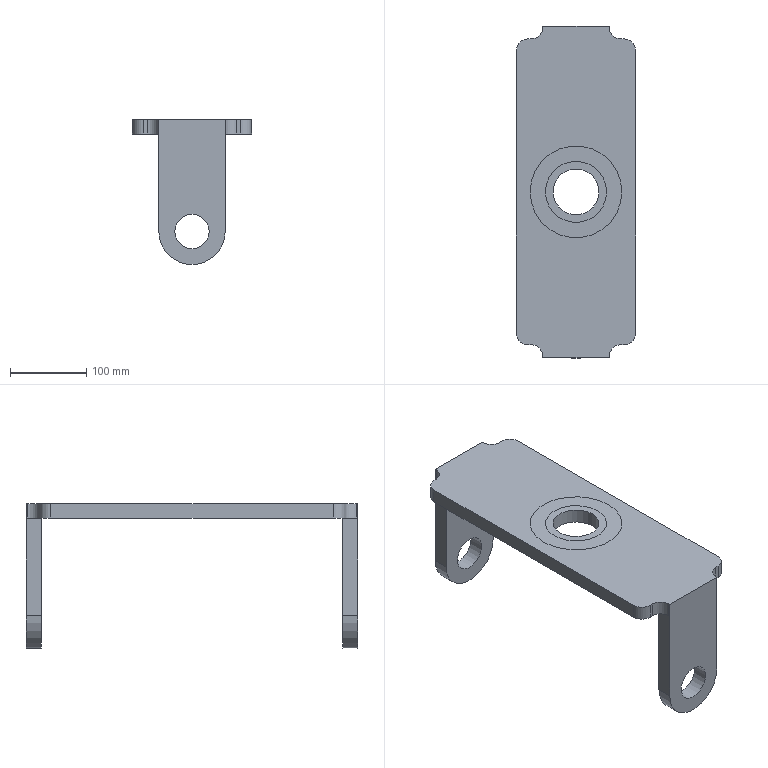Part | NX | features BREP 3 | 3 solids | 37 faces | box 156 x 434 x 190 mm | volume 1687057 mm3 | plane 20 | cylinder 17 | commonest cylinder face diameters 30 x8 45 x2 80 x2 87 x2 120 x2 60 x1
STEP:
#1=CARTESIAN_POINT('',(43.5,215.,19.));
#2=VERTEX_POINT('',#1);
#3=CARTESIAN_POINT('',(43.5,217.,19.));
#4=VERTEX_POINT('',#3);
#5=CARTESIAN_POINT('',(43.5,217.,19.));
#6=DIRECTION('',(0.,1.,0.));
#7=VECTOR('',#6,1000.);
#8=LINE('',#5,#7);
#9=EDGE_CURVE('',#2,#4,#8,.T.);
#10=ORIENTED_EDGE('',*,*,#9,.F.);
#11=CARTESIAN_POINT('',(43.5,215.,0.));
#12=VERTEX_POINT('',#11);
#13=CARTESIAN_POINT('',(43.5,215.,0.));
#14=DIRECTION('',(0.,0.,-1.));
#15=VECTOR('',#14,1000.);
#16=LINE('',#13,#15);
#17=EDGE_CURVE('',#2,#12,#16,.T.);
#18=ORIENTED_EDGE('',*,*,#17,.T.);
#19=CARTESIAN_POINT('',(43.5,197.,0.));
#20=VERTEX_POINT('',#19);
#21=CARTESIAN_POINT('',(43.5,217.,0.));
#22=DIRECTION('',(0.,-1.,0.));
#23=VECTOR('',#22,1000.);
#24=LINE('',#21,#23);
#25=EDGE_CURVE('',#12,#20,#24,.T.);
#26=ORIENTED_EDGE('',*,*,#25,.T.);
#27=CARTESIAN_POINT('',(43.5,197.,-127.5));
#28=VERTEX_POINT('',#27);
#29=CARTESIAN_POINT('',(43.5,197.,0.));
#30=DIRECTION('',(0.,0.,1.));
#31=VECTOR('',#30,1000.);
#32=LINE('',#29,#31);
#33=EDGE_CURVE('',#28,#20,#32,.T.);
#34=ORIENTED_EDGE('',*,*,#33,.F.);
#35=CARTESIAN_POINT('',(43.5,217.,-127.5));
#36=VERTEX_POINT('',#35);
#37=CARTESIAN_POINT('',(43.5,217.,-127.5));
#38=DIRECTION('',(0.,1.,0.));
#39=VECTOR('',#38,1000.);
#40=LINE('',#37,#39);
#41=EDGE_CURVE('',#28,#36,#40,.T.);
#42=ORIENTED_EDGE('',*,*,#41,.T.);
#43=CARTESIAN_POINT('',(43.5,217.,0.));
#44=DIRECTION('',(0.,0.,1.));
#45=VECTOR('',#44,1000.);
#46=LINE('',#43,#45);
#47=EDGE_CURVE('',#36,#4,#46,.T.);
#48=ORIENTED_EDGE('',*,*,#47,.T.);
#49=EDGE_LOOP('',(#10,#18,#26,#34,#42,#48));
#50=FACE_BOUND('',#49,.T.);
#51=CARTESIAN_POINT('',(43.5,217.,0.));
#52=DIRECTION('',(1.,0.,0.));
#53=DIRECTION('',(0.,0.,1.));
#54=AXIS2_PLACEMENT_3D('',#51,#52,#53);
#55=PLANE('',#54);
#56=ADVANCED_FACE('',(#50),#55,.T.);
#57=CARTESIAN_POINT('',(-43.5,197.,0.));
#58=VERTEX_POINT('',#57);
#59=CARTESIAN_POINT('',(-43.5,215.,0.));
#60=VERTEX_POINT('',#59);
#61=CARTESIAN_POINT('',(-43.5,217.,0.));
#62=DIRECTION('',(0.,1.,0.));
#63=VECTOR('',#62,1000.);
#64=LINE('',#61,#63);
#65=EDGE_CURVE('',#58,#60,#64,.T.);
#66=ORIENTED_EDGE('',*,*,#65,.T.);
#67=CARTESIAN_POINT('',(-43.5,215.,19.));
#68=VERTEX_POINT('',#67);
#69=CARTESIAN_POINT('',(-43.5,215.,-127.5));
#70=DIRECTION('',(0.,0.,1.));
#71=VECTOR('',#70,1000.);
#72=LINE('',#69,#71);
#73=EDGE_CURVE('',#60,#68,#72,.T.);
#74=ORIENTED_EDGE('',*,*,#73,.T.);
#75=CARTESIAN_POINT('',(-43.5,217.,19.));
#76=VERTEX_POINT('',#75);
#77=CARTESIAN_POINT('',(-43.5,217.,19.));
#78=DIRECTION('',(0.,1.,0.));
#79=VECTOR('',#78,1000.);
#80=LINE('',#77,#79);
#81=EDGE_CURVE('',#68,#76,#80,.T.);
#82=ORIENTED_EDGE('',*,*,#81,.T.);
#83=CARTESIAN_POINT('',(-43.5,217.,-127.5));
#84=VERTEX_POINT('',#83);
#85=CARTESIAN_POINT('',(-43.5,217.,-127.5));
#86=DIRECTION('',(0.,0.,-1.));
#87=VECTOR('',#86,1000.);
#88=LINE('',#85,#87);
#89=EDGE_CURVE('',#76,#84,#88,.T.);
#90=ORIENTED_EDGE('',*,*,#89,.T.);
#91=CARTESIAN_POINT('',(-43.5,197.,-127.5));
#92=VERTEX_POINT('',#91);
#93=CARTESIAN_POINT('',(-43.5,217.,-127.5));
#94=DIRECTION('',(0.,1.,0.));
#95=VECTOR('',#94,1000.);
#96=LINE('',#93,#95);
#97=EDGE_CURVE('',#92,#84,#96,.T.);
#98=ORIENTED_EDGE('',*,*,#97,.F.);
#99=CARTESIAN_POINT('',(-43.5,197.,-127.5));
#100=DIRECTION('',(0.,0.,-1.));
#101=VECTOR('',#100,1000.);
#102=LINE('',#99,#101);
#103=EDGE_CURVE('',#58,#92,#102,.T.);
#104=ORIENTED_EDGE('',*,*,#103,.F.);
#105=EDGE_LOOP('',(#66,#74,#82,#90,#98,#104));
#106=FACE_BOUND('',#105,.T.);
#107=CARTESIAN_POINT('',(-43.5,217.,-127.5));
#108=DIRECTION('',(-1.,0.,0.));
#109=DIRECTION('',(0.,0.,-1.));
#110=AXIS2_PLACEMENT_3D('',#107,#108,#109);
#111=PLANE('',#110);
#112=ADVANCED_FACE('',(#106),#111,.T.);
#113=CARTESIAN_POINT('',(22.5,197.,-127.5));
#114=VERTEX_POINT('',#113);
#115=CARTESIAN_POINT('',(0.,197.,-127.5));
#116=DIRECTION('',(0.,-1.,0.));
#117=DIRECTION('',(1.,0.,0.));
#118=AXIS2_PLACEMENT_3D('',#115,#116,#117);
#119=CIRCLE('',#118,22.5);
#120=EDGE_CURVE('',#114,#114,#119,.T.);
#121=ORIENTED_EDGE('',*,*,#120,.F.);
#122=EDGE_LOOP('',(#121));
#123=FACE_BOUND('',#122,.T.);
#124=ORIENTED_EDGE('',*,*,#33,.T.);
#125=CARTESIAN_POINT('',(0.,197.,0.));
#126=DIRECTION('',(-1.,0.,0.));
#127=VECTOR('',#126,1000.);
#128=LINE('',#125,#127);
#129=EDGE_CURVE('',#20,#58,#128,.T.);
#130=ORIENTED_EDGE('',*,*,#129,.T.);
#131=ORIENTED_EDGE('',*,*,#103,.T.);
#132=CARTESIAN_POINT('',(0.,197.,-127.5));
#133=DIRECTION('',(0.,-1.,0.));
#134=DIRECTION('',(1.,0.,0.));
#135=AXIS2_PLACEMENT_3D('',#132,#133,#134);
#136=CIRCLE('',#135,43.5);
#137=EDGE_CURVE('',#92,#28,#136,.T.);
#138=ORIENTED_EDGE('',*,*,#137,.T.);
#139=EDGE_LOOP('',(#124,#130,#131,#138));
#140=FACE_BOUND('',#139,.T.);
#141=CARTESIAN_POINT('',(0.,197.,-127.5));
#142=DIRECTION('',(0.,-1.,0.));
#143=DIRECTION('',(0.,0.,-1.));
#144=AXIS2_PLACEMENT_3D('',#141,#142,#143);
#145=PLANE('',#144);
#146=ADVANCED_FACE('',(#123,#140),#145,.T.);
#147=ORIENTED_EDGE('',*,*,#137,.F.);
#148=ORIENTED_EDGE('',*,*,#97,.T.);
#149=CARTESIAN_POINT('',(0.,217.,-127.5));
#150=DIRECTION('',(0.,-1.,0.));
#151=DIRECTION('',(1.,0.,0.));
#152=AXIS2_PLACEMENT_3D('',#149,#150,#151);
#153=CIRCLE('',#152,43.5);
#154=EDGE_CURVE('',#84,#36,#153,.T.);
#155=ORIENTED_EDGE('',*,*,#154,.T.);
#156=ORIENTED_EDGE('',*,*,#41,.F.);
#157=EDGE_LOOP('',(#147,#148,#155,#156));
#158=FACE_BOUND('',#157,.T.);
#159=CARTESIAN_POINT('',(0.,217.,-127.5));
#160=DIRECTION('',(0.,-1.,0.));
#161=DIRECTION('',(0.,0.,-1.));
#162=AXIS2_PLACEMENT_3D('',#159,#160,#161);
#163=CYLINDRICAL_SURFACE('',#162,43.5);
#164=ADVANCED_FACE('',(#158),#163,.T.);
#165=CARTESIAN_POINT('',(60.,0.,19.));
#166=VERTEX_POINT('',#165);
#167=CARTESIAN_POINT('',(0.,0.,19.));
#168=DIRECTION('',(0.,0.,1.));
#169=DIRECTION('',(1.,0.,0.));
#170=AXIS2_PLACEMENT_3D('',#167,#168,#169);
#171=CIRCLE('',#170,60.);
#172=EDGE_CURVE('',#166,#166,#171,.T.);
#173=ORIENTED_EDGE('',*,*,#172,.F.);
#174=EDGE_LOOP('',(#173));
#175=FACE_BOUND('',#174,.T.);
#176=CARTESIAN_POINT('',(-78.,185.,19.));
#177=VERTEX_POINT('',#176);
#178=CARTESIAN_POINT('',(-78.,-185.,19.));
#179=VERTEX_POINT('',#178);
#180=CARTESIAN_POINT('',(-78.,175.,19.));
#181=DIRECTION('',(0.,-1.,0.));
#182=VECTOR('',#181,1000.);
#183=LINE('',#180,#182);
#184=EDGE_CURVE('',#177,#179,#183,.T.);
#185=ORIENTED_EDGE('',*,*,#184,.T.);
#186=CARTESIAN_POINT('',(-63.,-200.,19.));
#187=VERTEX_POINT('',#186);
#188=CARTESIAN_POINT('',(-63.,-185.,19.));
#189=DIRECTION('',(0.,0.,1.));
#190=DIRECTION('',(1.,0.,0.));
#191=AXIS2_PLACEMENT_3D('',#188,#189,#190);
#192=CIRCLE('',#191,15.);
#193=EDGE_CURVE('',#179,#187,#192,.T.);
#194=ORIENTED_EDGE('',*,*,#193,.T.);
#195=CARTESIAN_POINT('',(-58.5,-200.,19.));
#196=VERTEX_POINT('',#195);
#197=CARTESIAN_POINT('',(-48.,-200.,19.));
#198=DIRECTION('',(1.,0.,0.));
#199=VECTOR('',#198,1000.);
#200=LINE('',#197,#199);
#201=EDGE_CURVE('',#187,#196,#200,.T.);
#202=ORIENTED_EDGE('',*,*,#201,.T.);
#203=CARTESIAN_POINT('',(-43.5,-215.,19.));
#204=VERTEX_POINT('',#203);
#205=CARTESIAN_POINT('',(-58.5,-215.,19.));
#206=DIRECTION('',(0.,0.,-1.));
#207=DIRECTION('',(1.,0.,0.));
#208=AXIS2_PLACEMENT_3D('',#205,#206,#207);
#209=CIRCLE('',#208,15.);
#210=EDGE_CURVE('',#196,#204,#209,.T.);
#211=ORIENTED_EDGE('',*,*,#210,.T.);
#212=CARTESIAN_POINT('',(-43.5,-217.,19.));
#213=VERTEX_POINT('',#212);
#214=CARTESIAN_POINT('',(-43.5,-217.,19.));
#215=DIRECTION('',(0.,1.,0.));
#216=VECTOR('',#215,1000.);
#217=LINE('',#214,#216);
#218=EDGE_CURVE('',#213,#204,#217,.T.);
#219=ORIENTED_EDGE('',*,*,#218,.F.);
#220=CARTESIAN_POINT('',(43.5,-217.,19.));
#221=VERTEX_POINT('',#220);
#222=CARTESIAN_POINT('',(0.,-217.,19.));
#223=DIRECTION('',(1.,0.,0.));
#224=VECTOR('',#223,1000.);
#225=LINE('',#222,#224);
#226=EDGE_CURVE('',#213,#221,#225,.T.);
#227=ORIENTED_EDGE('',*,*,#226,.T.);
#228=CARTESIAN_POINT('',(43.5,-215.,19.));
#229=VERTEX_POINT('',#228);
#230=CARTESIAN_POINT('',(43.5,-217.,19.));
#231=DIRECTION('',(0.,1.,0.));
#232=VECTOR('',#231,1000.);
#233=LINE('',#230,#232);
#234=EDGE_CURVE('',#221,#229,#233,.T.);
#235=ORIENTED_EDGE('',*,*,#234,.T.);
#236=CARTESIAN_POINT('',(58.5,-200.,19.));
#237=VERTEX_POINT('',#236);
#238=CARTESIAN_POINT('',(58.5,-215.,19.));
#239=DIRECTION('',(0.,0.,-1.));
#240=DIRECTION('',(1.,0.,0.));
#241=AXIS2_PLACEMENT_3D('',#238,#239,#240);
#242=CIRCLE('',#241,15.);
#243=EDGE_CURVE('',#229,#237,#242,.T.);
#244=ORIENTED_EDGE('',*,*,#243,.T.);
#245=CARTESIAN_POINT('',(63.,-200.,19.));
#246=VERTEX_POINT('',#245);
#247=CARTESIAN_POINT('',(-48.,-200.,19.));
#248=DIRECTION('',(1.,0.,0.));
#249=VECTOR('',#248,1000.);
#250=LINE('',#247,#249);
#251=EDGE_CURVE('',#237,#246,#250,.T.);
#252=ORIENTED_EDGE('',*,*,#251,.T.);
#253=CARTESIAN_POINT('',(78.,-185.,19.));
#254=VERTEX_POINT('',#253);
#255=CARTESIAN_POINT('',(63.,-185.,19.));
#256=DIRECTION('',(0.,0.,1.));
#257=DIRECTION('',(1.,0.,0.));
#258=AXIS2_PLACEMENT_3D('',#255,#256,#257);
#259=CIRCLE('',#258,15.);
#260=EDGE_CURVE('',#246,#254,#259,.T.);
#261=ORIENTED_EDGE('',*,*,#260,.T.);
#262=CARTESIAN_POINT('',(78.,185.,19.));
#263=VERTEX_POINT('',#262);
#264=CARTESIAN_POINT('',(78.,-175.,19.));
#265=DIRECTION('',(0.,1.,0.));
#266=VECTOR('',#265,1000.);
#267=LINE('',#264,#266);
#268=EDGE_CURVE('',#254,#263,#267,.T.);
#269=ORIENTED_EDGE('',*,*,#268,.T.);
#270=CARTESIAN_POINT('',(63.,200.,19.));
#271=VERTEX_POINT('',#270);
#272=CARTESIAN_POINT('',(63.,185.,19.));
#273=DIRECTION('',(0.,0.,1.));
#274=DIRECTION('',(1.,0.,0.));
#275=AXIS2_PLACEMENT_3D('',#272,#273,#274);
#276=CIRCLE('',#275,15.);
#277=EDGE_CURVE('',#263,#271,#276,.T.);
#278=ORIENTED_EDGE('',*,*,#277,.T.);
#279=CARTESIAN_POINT('',(58.5,200.,19.));
#280=VERTEX_POINT('',#279);
#281=CARTESIAN_POINT('',(-48.,200.,19.));
#282=DIRECTION('',(-1.,0.,0.));
#283=VECTOR('',#282,1000.);
#284=LINE('',#281,#283);
#285=EDGE_CURVE('',#271,#280,#284,.T.);
#286=ORIENTED_EDGE('',*,*,#285,.T.);
#287=CARTESIAN_POINT('',(58.5,215.,19.));
#288=DIRECTION('',(0.,0.,-1.));
#289=DIRECTION('',(1.,0.,0.));
#290=AXIS2_PLACEMENT_3D('',#287,#288,#289);
#291=CIRCLE('',#290,15.);
#292=EDGE_CURVE('',#280,#2,#291,.T.);
#293=ORIENTED_EDGE('',*,*,#292,.T.);
#294=ORIENTED_EDGE('',*,*,#9,.T.);
#295=CARTESIAN_POINT('',(0.,217.,19.));
#296=DIRECTION('',(-1.,0.,0.));
#297=VECTOR('',#296,1000.);
#298=LINE('',#295,#297);
#299=EDGE_CURVE('',#4,#76,#298,.T.);
#300=ORIENTED_EDGE('',*,*,#299,.T.);
#301=ORIENTED_EDGE('',*,*,#81,.F.);
#302=CARTESIAN_POINT('',(-58.5,200.,19.));
#303=VERTEX_POINT('',#302);
#304=CARTESIAN_POINT('',(-58.5,215.,19.));
#305=DIRECTION('',(0.,0.,-1.));
#306=DIRECTION('',(1.,0.,0.));
#307=AXIS2_PLACEMENT_3D('',#304,#305,#306);
#308=CIRCLE('',#307,15.);
#309=EDGE_CURVE('',#68,#303,#308,.T.);
#310=ORIENTED_EDGE('',*,*,#309,.T.);
#311=CARTESIAN_POINT('',(-63.,200.,19.));
#312=VERTEX_POINT('',#311);
#313=CARTESIAN_POINT('',(-48.,200.,19.));
#314=DIRECTION('',(-1.,0.,0.));
#315=VECTOR('',#314,1000.);
#316=LINE('',#313,#315);
#317=EDGE_CURVE('',#303,#312,#316,.T.);
#318=ORIENTED_EDGE('',*,*,#317,.T.);
#319=CARTESIAN_POINT('',(-63.,185.,19.));
#320=DIRECTION('',(0.,0.,1.));
#321=DIRECTION('',(1.,0.,0.));
#322=AXIS2_PLACEMENT_3D('',#319,#320,#321);
#323=CIRCLE('',#322,15.);
#324=EDGE_CURVE('',#312,#177,#323,.T.);
#325=ORIENTED_EDGE('',*,*,#324,.T.);
#326=EDGE_LOOP('',(#185,#194,#202,#211,#219,#227,#235,#244,#252,#261,#269,#278,#286,#293,#294,#300,#301,#310,#318,#325));
#327=FACE_BOUND('',#326,.T.);
#328=CARTESIAN_POINT('',(-43.5,217.,19.));
#329=DIRECTION('',(0.,0.,1.));
#330=DIRECTION('',(-1.,0.,0.));
#331=AXIS2_PLACEMENT_3D('',#328,#329,#330);
#332=PLANE('',#331);
#333=ADVANCED_FACE('',(#175,#327),#332,.T.);
#334=CARTESIAN_POINT('',(22.5,217.,-127.5));
#335=VERTEX_POINT('',#334);
#336=CARTESIAN_POINT('',(0.,217.,-127.5));
#337=DIRECTION('',(0.,-1.,0.));
#338=DIRECTION('',(1.,0.,0.));
#339=AXIS2_PLACEMENT_3D('',#336,#337,#338);
#340=CIRCLE('',#339,22.5);
#341=EDGE_CURVE('',#335,#335,#340,.T.);
#342=ORIENTED_EDGE('',*,*,#341,.F.);
#343=EDGE_LOOP('',(#342));
#344=FACE_BOUND('',#343,.T.);
#345=ORIENTED_EDGE('',*,*,#120,.T.);
#346=EDGE_LOOP('',(#345));
#347=FACE_BOUND('',#346,.T.);
#348=CARTESIAN_POINT('',(0.,217.,-127.5));
#349=DIRECTION('',(0.,-1.,0.));
#350=DIRECTION('',(0.,0.,-1.));
#351=AXIS2_PLACEMENT_3D('',#348,#349,#350);
#352=CYLINDRICAL_SURFACE('',#351,22.5);
#353=ADVANCED_FACE('',(#344,#347),#352,.F.);
#354=ORIENTED_EDGE('',*,*,#47,.F.);
#355=ORIENTED_EDGE('',*,*,#154,.F.);
#356=ORIENTED_EDGE('',*,*,#89,.F.);
#357=ORIENTED_EDGE('',*,*,#299,.F.);
#358=EDGE_LOOP('',(#354,#355,#356,#357));
#359=FACE_BOUND('',#358,.T.);
#360=ORIENTED_EDGE('',*,*,#341,.T.);
#361=EDGE_LOOP('',(#360));
#362=FACE_BOUND('',#361,.T.);
#363=CARTESIAN_POINT('',(0.,217.,-127.5));
#364=DIRECTION('',(0.,-1.,0.));
#365=DIRECTION('',(0.,0.,-1.));
#366=AXIS2_PLACEMENT_3D('',#363,#364,#365);
#367=PLANE('',#366);
#368=ADVANCED_FACE('',(#359,#362),#367,.F.);
#369=ORIENTED_EDGE('',*,*,#285,.F.);
#370=CARTESIAN_POINT('',(63.,200.,0.));
#371=VERTEX_POINT('',#370);
#372=CARTESIAN_POINT('',(63.,200.,19.));
#373=DIRECTION('',(0.,0.,-1.));
#374=VECTOR('',#373,1000.);
#375=LINE('',#372,#374);
#376=EDGE_CURVE('',#271,#371,#375,.T.);
#377=ORIENTED_EDGE('',*,*,#376,.T.);
#378=CARTESIAN_POINT('',(58.5,200.,0.));
#379=VERTEX_POINT('',#378);
#380=CARTESIAN_POINT('',(-48.,200.,0.));
#381=DIRECTION('',(-1.,0.,0.));
#382=VECTOR('',#381,1000.);
#383=LINE('',#380,#382);
#384=EDGE_CURVE('',#371,#379,#383,.T.);
#385=ORIENTED_EDGE('',*,*,#384,.T.);
#386=CARTESIAN_POINT('',(58.5,200.,19.));
#387=DIRECTION('',(0.,0.,1.));
#388=VECTOR('',#387,1000.);
#389=LINE('',#386,#388);
#390=EDGE_CURVE('',#379,#280,#389,.T.);
#391=ORIENTED_EDGE('',*,*,#390,.T.);
#392=EDGE_LOOP('',(#369,#377,#385,#391));
#393=FACE_BOUND('',#392,.T.);
#394=CARTESIAN_POINT('',(-48.,200.,19.));
#395=DIRECTION('',(0.,-1.,0.));
#396=DIRECTION('',(-1.,0.,0.));
#397=AXIS2_PLACEMENT_3D('',#394,#395,#396);
#398=PLANE('',#397);
#399=ADVANCED_FACE('',(#393),#398,.F.);
#400=CARTESIAN_POINT('',(58.5,-200.,0.));
#401=VERTEX_POINT('',#400);
#402=CARTESIAN_POINT('',(63.,-200.,0.));
#403=VERTEX_POINT('',#402);
#404=CARTESIAN_POINT('',(-48.,-200.,0.));
#405=DIRECTION('',(1.,0.,0.));
#406=VECTOR('',#405,1000.);
#407=LINE('',#404,#406);
#408=EDGE_CURVE('',#401,#403,#407,.T.);
#409=ORIENTED_EDGE('',*,*,#408,.T.);
#410=CARTESIAN_POINT('',(63.,-200.,19.));
#411=DIRECTION('',(0.,0.,1.));
#412=VECTOR('',#411,1000.);
#413=LINE('',#410,#412);
#414=EDGE_CURVE('',#403,#246,#413,.T.);
#415=ORIENTED_EDGE('',*,*,#414,.T.);
#416=ORIENTED_EDGE('',*,*,#251,.F.);
#417=CARTESIAN_POINT('',(58.5,-200.,19.));
#418=DIRECTION('',(0.,0.,-1.));
#419=VECTOR('',#418,1000.);
#420=LINE('',#417,#419);
#421=EDGE_CURVE('',#237,#401,#420,.T.);
#422=ORIENTED_EDGE('',*,*,#421,.T.);
#423=EDGE_LOOP('',(#409,#415,#416,#422));
#424=FACE_BOUND('',#423,.T.);
#425=CARTESIAN_POINT('',(-48.,-200.,19.));
#426=DIRECTION('',(0.,1.,0.));
#427=DIRECTION('',(0.,0.,-1.));
#428=AXIS2_PLACEMENT_3D('',#425,#426,#427);
#429=PLANE('',#428);
#430=ADVANCED_FACE('',(#424),#429,.F.);
#431=ORIENTED_EDGE('',*,*,#268,.F.);
#432=CARTESIAN_POINT('',(78.,-185.,0.));
#433=VERTEX_POINT('',#432);
#434=CARTESIAN_POINT('',(78.,-185.,19.));
#435=DIRECTION('',(0.,0.,-1.));
#436=VECTOR('',#435,1000.);
#437=LINE('',#434,#436);
#438=EDGE_CURVE('',#254,#433,#437,.T.);
#439=ORIENTED_EDGE('',*,*,#438,.T.);
#440=CARTESIAN_POINT('',(78.,185.,0.));
#441=VERTEX_POINT('',#440);
#442=CARTESIAN_POINT('',(78.,-175.,0.));
#443=DIRECTION('',(0.,1.,0.));
#444=VECTOR('',#443,1000.);
#445=LINE('',#442,#444);
#446=EDGE_CURVE('',#433,#441,#445,.T.);
#447=ORIENTED_EDGE('',*,*,#446,.T.);
#448=CARTESIAN_POINT('',(78.,185.,19.));
#449=DIRECTION('',(0.,0.,1.));
#450=VECTOR('',#449,1000.);
#451=LINE('',#448,#450);
#452=EDGE_CURVE('',#441,#263,#451,.T.);
#453=ORIENTED_EDGE('',*,*,#452,.T.);
#454=EDGE_LOOP('',(#431,#439,#447,#453));
#455=FACE_BOUND('',#454,.T.);
#456=CARTESIAN_POINT('',(78.,-175.,19.));
#457=DIRECTION('',(-1.,0.,0.));
#458=DIRECTION('',(0.,1.,0.));
#459=AXIS2_PLACEMENT_3D('',#456,#457,#458);
#460=PLANE('',#459);
#461=ADVANCED_FACE('',(#455),#460,.F.);
#462=CARTESIAN_POINT('',(-58.5,200.,0.));
#463=VERTEX_POINT('',#462);
#464=CARTESIAN_POINT('',(-63.,200.,0.));
#465=VERTEX_POINT('',#464);
#466=CARTESIAN_POINT('',(-48.,200.,0.));
#467=DIRECTION('',(-1.,0.,0.));
#468=VECTOR('',#467,1000.);
#469=LINE('',#466,#468);
#470=EDGE_CURVE('',#463,#465,#469,.T.);
#471=ORIENTED_EDGE('',*,*,#470,.T.);
#472=CARTESIAN_POINT('',(-63.,200.,19.));
#473=DIRECTION('',(0.,0.,1.));
#474=VECTOR('',#473,1000.);
#475=LINE('',#472,#474);
#476=EDGE_CURVE('',#465,#312,#475,.T.);
#477=ORIENTED_EDGE('',*,*,#476,.T.);
#478=ORIENTED_EDGE('',*,*,#317,.F.);
#479=CARTESIAN_POINT('',(-58.5,200.,19.));
#480=DIRECTION('',(0.,0.,-1.));
#481=VECTOR('',#480,1000.);
#482=LINE('',#479,#481);
#483=EDGE_CURVE('',#303,#463,#482,.T.);
#484=ORIENTED_EDGE('',*,*,#483,.T.);
#485=EDGE_LOOP('',(#471,#477,#478,#484));
#486=FACE_BOUND('',#485,.T.);
#487=CARTESIAN_POINT('',(-48.,200.,19.));
#488=DIRECTION('',(0.,-1.,0.));
#489=DIRECTION('',(-1.,0.,0.));
#490=AXIS2_PLACEMENT_3D('',#487,#488,#489);
#491=PLANE('',#490);
#492=ADVANCED_FACE('',(#486),#491,.F.);
#493=CARTESIAN_POINT('',(-78.,185.,0.));
#494=VERTEX_POINT('',#493);
#495=CARTESIAN_POINT('',(-78.,-185.,0.));
#496=VERTEX_POINT('',#495);
#497=CARTESIAN_POINT('',(-78.,175.,0.));
#498=DIRECTION('',(0.,-1.,0.));
#499=VECTOR('',#498,1000.);
#500=LINE('',#497,#499);
#501=EDGE_CURVE('',#494,#496,#500,.T.);
#502=ORIENTED_EDGE('',*,*,#501,.T.);
#503=CARTESIAN_POINT('',(-78.,-185.,19.));
#504=DIRECTION('',(0.,0.,1.));
#505=VECTOR('',#504,1000.);
#506=LINE('',#503,#505);
#507=EDGE_CURVE('',#496,#179,#506,.T.);
#508=ORIENTED_EDGE('',*,*,#507,.T.);
#509=ORIENTED_EDGE('',*,*,#184,.F.);
#510=CARTESIAN_POINT('',(-78.,185.,19.));
#511=DIRECTION('',(0.,0.,-1.));
#512=VECTOR('',#511,1000.);
#513=LINE('',#510,#512);
#514=EDGE_CURVE('',#177,#494,#513,.T.);
#515=ORIENTED_EDGE('',*,*,#514,.T.);
#516=EDGE_LOOP('',(#502,#508,#509,#515));
#517=FACE_BOUND('',#516,.T.);
#518=CARTESIAN_POINT('',(-78.,175.,19.));
#519=DIRECTION('',(1.,0.,0.));
#520=DIRECTION('',(0.,0.,1.));
#521=AXIS2_PLACEMENT_3D('',#518,#519,#520);
#522=PLANE('',#521);
#523=ADVANCED_FACE('',(#517),#522,.F.);
#524=ORIENTED_EDGE('',*,*,#201,.F.);
#525=CARTESIAN_POINT('',(-63.,-200.,0.));
#526=VERTEX_POINT('',#525);
#527=CARTESIAN_POINT('',(-63.,-200.,19.));
#528=DIRECTION('',(0.,0.,-1.));
#529=VECTOR('',#528,1000.);
#530=LINE('',#527,#529);
#531=EDGE_CURVE('',#187,#526,#530,.T.);
#532=ORIENTED_EDGE('',*,*,#531,.T.);
#533=CARTESIAN_POINT('',(-58.5,-200.,0.));
#534=VERTEX_POINT('',#533);
#535=CARTESIAN_POINT('',(-48.,-200.,0.));
#536=DIRECTION('',(1.,0.,0.));
#537=VECTOR('',#536,1000.);
#538=LINE('',#535,#537);
#539=EDGE_CURVE('',#526,#534,#538,.T.);
#540=ORIENTED_EDGE('',*,*,#539,.T.);
#541=CARTESIAN_POINT('',(-58.5,-200.,19.));
#542=DIRECTION('',(0.,0.,1.));
#543=VECTOR('',#542,1000.);
#544=LINE('',#541,#543);
#545=EDGE_CURVE('',#534,#196,#544,.T.);
#546=ORIENTED_EDGE('',*,*,#545,.T.);
#547=EDGE_LOOP('',(#524,#532,#540,#546));
#548=FACE_BOUND('',#547,.T.);
#549=CARTESIAN_POINT('',(-48.,-200.,19.));
#550=DIRECTION('',(0.,1.,0.));
#551=DIRECTION('',(0.,0.,-1.));
#552=AXIS2_PLACEMENT_3D('',#549,#550,#551);
#553=PLANE('',#552);
#554=ADVANCED_FACE('',(#548),#553,.F.);
#555=CARTESIAN_POINT('',(60.,0.,0.));
#556=VERTEX_POINT('',#555);
#557=CARTESIAN_POINT('',(0.,0.,0.));
#558=DIRECTION('',(0.,0.,1.));
#559=DIRECTION('',(1.,0.,0.));
#560=AXIS2_PLACEMENT_3D('',#557,#558,#559);
#561=CIRCLE('',#560,60.);
#562=EDGE_CURVE('',#556,#556,#561,.T.);
#563=ORIENTED_EDGE('',*,*,#562,.T.);
#564=EDGE_LOOP('',(#563));
#565=FACE_BOUND('',#564,.T.);
#566=ORIENTED_EDGE('',*,*,#539,.F.);
#567=CARTESIAN_POINT('',(-63.,-185.,0.));
#568=DIRECTION('',(0.,0.,-1.));
#569=DIRECTION('',(1.,0.,0.));
#570=AXIS2_PLACEMENT_3D('',#567,#568,#569);
#571=CIRCLE('',#570,15.);
#572=EDGE_CURVE('',#526,#496,#571,.T.);
#573=ORIENTED_EDGE('',*,*,#572,.T.);
#574=ORIENTED_EDGE('',*,*,#501,.F.);
#575=CARTESIAN_POINT('',(-63.,185.,0.));
#576=DIRECTION('',(0.,0.,-1.));
#577=DIRECTION('',(1.,0.,0.));
#578=AXIS2_PLACEMENT_3D('',#575,#576,#577);
#579=CIRCLE('',#578,15.);
#580=EDGE_CURVE('',#494,#465,#579,.T.);
#581=ORIENTED_EDGE('',*,*,#580,.T.);
#582=ORIENTED_EDGE('',*,*,#470,.F.);
#583=CARTESIAN_POINT('',(-58.5,215.,0.));
#584=DIRECTION('',(0.,0.,1.));
#585=DIRECTION('',(1.,0.,0.));
#586=AXIS2_PLACEMENT_3D('',#583,#584,#585);
#587=CIRCLE('',#586,15.);
#588=EDGE_CURVE('',#463,#60,#587,.T.);
#589=ORIENTED_EDGE('',*,*,#588,.T.);
#590=ORIENTED_EDGE('',*,*,#65,.F.);
#591=ORIENTED_EDGE('',*,*,#129,.F.);
#592=ORIENTED_EDGE('',*,*,#25,.F.);
#593=CARTESIAN_POINT('',(58.5,215.,0.));
#594=DIRECTION('',(0.,0.,1.));
#595=DIRECTION('',(1.,0.,0.));
#596=AXIS2_PLACEMENT_3D('',#593,#594,#595);
#597=CIRCLE('',#596,15.);
#598=EDGE_CURVE('',#12,#379,#597,.T.);
#599=ORIENTED_EDGE('',*,*,#598,.T.);
#600=ORIENTED_EDGE('',*,*,#384,.F.);
#601=CARTESIAN_POINT('',(63.,185.,0.));
#602=DIRECTION('',(0.,0.,-1.));
#603=DIRECTION('',(1.,0.,0.));
#604=AXIS2_PLACEMENT_3D('',#601,#602,#603);
#605=CIRCLE('',#604,15.);
#606=EDGE_CURVE('',#371,#441,#605,.T.);
#607=ORIENTED_EDGE('',*,*,#606,.T.);
#608=ORIENTED_EDGE('',*,*,#446,.F.);
#609=CARTESIAN_POINT('',(63.,-185.,0.));
#610=DIRECTION('',(0.,0.,-1.));
#611=DIRECTION('',(1.,0.,0.));
#612=AXIS2_PLACEMENT_3D('',#609,#610,#611);
#613=CIRCLE('',#612,15.);
#614=EDGE_CURVE('',#433,#403,#613,.T.);
#615=ORIENTED_EDGE('',*,*,#614,.T.);
#616=ORIENTED_EDGE('',*,*,#408,.F.);
#617=CARTESIAN_POINT('',(43.5,-215.,0.));
#618=VERTEX_POINT('',#617);
#619=CARTESIAN_POINT('',(58.5,-215.,0.));
#620=DIRECTION('',(0.,0.,1.));
#621=DIRECTION('',(1.,0.,0.));
#622=AXIS2_PLACEMENT_3D('',#619,#620,#621);
#623=CIRCLE('',#622,15.);
#624=EDGE_CURVE('',#401,#618,#623,.T.);
#625=ORIENTED_EDGE('',*,*,#624,.T.);
#626=CARTESIAN_POINT('',(43.5,-197.,0.));
#627=VERTEX_POINT('',#626);
#628=CARTESIAN_POINT('',(43.5,0.,0.));
#629=DIRECTION('',(0.,1.,0.));
#630=VECTOR('',#629,1000.);
#631=LINE('',#628,#630);
#632=EDGE_CURVE('',#618,#627,#631,.T.);
#633=ORIENTED_EDGE('',*,*,#632,.T.);
#634=CARTESIAN_POINT('',(-43.5,-197.,0.));
#635=VERTEX_POINT('',#634);
#636=CARTESIAN_POINT('',(0.,-197.,0.));
#637=DIRECTION('',(-1.,0.,0.));
#638=VECTOR('',#637,1000.);
#639=LINE('',#636,#638);
#640=EDGE_CURVE('',#627,#635,#639,.T.);
#641=ORIENTED_EDGE('',*,*,#640,.T.);
#642=CARTESIAN_POINT('',(-43.5,-215.,0.));
#643=VERTEX_POINT('',#642);
#644=CARTESIAN_POINT('',(-43.5,0.,0.));
#645=DIRECTION('',(0.,-1.,0.));
#646=VECTOR('',#645,1000.);
#647=LINE('',#644,#646);
#648=EDGE_CURVE('',#635,#643,#647,.T.);
#649=ORIENTED_EDGE('',*,*,#648,.T.);
#650=CARTESIAN_POINT('',(-58.5,-215.,0.));
#651=DIRECTION('',(0.,0.,1.));
#652=DIRECTION('',(1.,0.,0.));
#653=AXIS2_PLACEMENT_3D('',#650,#651,#652);
#654=CIRCLE('',#653,15.);
#655=EDGE_CURVE('',#643,#534,#654,.T.);
#656=ORIENTED_EDGE('',*,*,#655,.T.);
#657=EDGE_LOOP('',(#566,#573,#574,#581,#582,#589,#590,#591,#592,#599,#600,#607,#608,#615,#616,#625,#633,#641,#649,#656));
#658=FACE_BOUND('',#657,.T.);
#659=CARTESIAN_POINT('',(0.,0.,0.));
#660=DIRECTION('',(0.,0.,1.));
#661=DIRECTION('',(-1.,0.,0.));
#662=AXIS2_PLACEMENT_3D('',#659,#660,#661);
#663=PLANE('',#662);
#664=ADVANCED_FACE('',(#565,#658),#663,.F.);
#665=ORIENTED_EDGE('',*,*,#632,.F.);
#666=CARTESIAN_POINT('',(43.5,-215.,0.));
#667=DIRECTION('',(0.,0.,1.));
#668=VECTOR('',#667,1000.);
#669=LINE('',#666,#668);
#670=EDGE_CURVE('',#618,#229,#669,.T.);
#671=ORIENTED_EDGE('',*,*,#670,.T.);
#672=ORIENTED_EDGE('',*,*,#234,.F.);
#673=CARTESIAN_POINT('',(43.5,-217.,-127.5));
#674=VERTEX_POINT('',#673);
#675=CARTESIAN_POINT('',(43.5,-217.,0.));
#676=DIRECTION('',(0.,0.,-1.));
#677=VECTOR('',#676,1000.);
#678=LINE('',#675,#677);
#679=EDGE_CURVE('',#221,#674,#678,.T.);
#680=ORIENTED_EDGE('',*,*,#679,.T.);
#681=CARTESIAN_POINT('',(43.5,-197.,-127.5));
#682=VERTEX_POINT('',#681);
#683=CARTESIAN_POINT('',(43.5,-217.,-127.5));
#684=DIRECTION('',(0.,1.,0.));
#685=VECTOR('',#684,1000.);
#686=LINE('',#683,#685);
#687=EDGE_CURVE('',#674,#682,#686,.T.);
#688=ORIENTED_EDGE('',*,*,#687,.T.);
#689=CARTESIAN_POINT('',(43.5,-197.,0.));
#690=DIRECTION('',(0.,0.,-1.));
#691=VECTOR('',#690,1000.);
#692=LINE('',#689,#691);
#693=EDGE_CURVE('',#627,#682,#692,.T.);
#694=ORIENTED_EDGE('',*,*,#693,.F.);
#695=EDGE_LOOP('',(#665,#671,#672,#680,#688,#694));
#696=FACE_BOUND('',#695,.T.);
#697=CARTESIAN_POINT('',(43.5,-217.,0.));
#698=DIRECTION('',(1.,0.,0.));
#699=DIRECTION('',(0.,0.,1.));
#700=AXIS2_PLACEMENT_3D('',#697,#698,#699);
#701=PLANE('',#700);
#702=ADVANCED_FACE('',(#696),#701,.T.);
#703=ORIENTED_EDGE('',*,*,#218,.T.);
#704=CARTESIAN_POINT('',(-43.5,-215.,-127.5));
#705=DIRECTION('',(0.,0.,-1.));
#706=VECTOR('',#705,1000.);
#707=LINE('',#704,#706);
#708=EDGE_CURVE('',#204,#643,#707,.T.);
#709=ORIENTED_EDGE('',*,*,#708,.T.);
#710=ORIENTED_EDGE('',*,*,#648,.F.);
#711=CARTESIAN_POINT('',(-43.5,-197.,-127.5));
#712=VERTEX_POINT('',#711);
#713=CARTESIAN_POINT('',(-43.5,-197.,-127.5));
#714=DIRECTION('',(0.,0.,1.));
#715=VECTOR('',#714,1000.);
#716=LINE('',#713,#715);
#717=EDGE_CURVE('',#712,#635,#716,.T.);
#718=ORIENTED_EDGE('',*,*,#717,.F.);
#719=CARTESIAN_POINT('',(-43.5,-217.,-127.5));
#720=VERTEX_POINT('',#719);
#721=CARTESIAN_POINT('',(-43.5,-217.,-127.5));
#722=DIRECTION('',(0.,1.,0.));
#723=VECTOR('',#722,1000.);
#724=LINE('',#721,#723);
#725=EDGE_CURVE('',#720,#712,#724,.T.);
#726=ORIENTED_EDGE('',*,*,#725,.F.);
#727=CARTESIAN_POINT('',(-43.5,-217.,-127.5));
#728=DIRECTION('',(0.,0.,1.));
#729=VECTOR('',#728,1000.);
#730=LINE('',#727,#729);
#731=EDGE_CURVE('',#720,#213,#730,.T.);
#732=ORIENTED_EDGE('',*,*,#731,.T.);
#733=EDGE_LOOP('',(#703,#709,#710,#718,#726,#732));
#734=FACE_BOUND('',#733,.T.);
#735=CARTESIAN_POINT('',(-43.5,-217.,-127.5));
#736=DIRECTION('',(-1.,0.,0.));
#737=DIRECTION('',(0.,0.,-1.));
#738=AXIS2_PLACEMENT_3D('',#735,#736,#737);
#739=PLANE('',#738);
#740=ADVANCED_FACE('',(#734),#739,.T.);
#741=CARTESIAN_POINT('',(22.5,-197.,-127.5));
#742=VERTEX_POINT('',#741);
#743=CARTESIAN_POINT('',(0.,-197.,-127.5));
#744=DIRECTION('',(0.,1.,0.));
#745=DIRECTION('',(1.,0.,0.));
#746=AXIS2_PLACEMENT_3D('',#743,#744,#745);
#747=CIRCLE('',#746,22.5);
#748=EDGE_CURVE('',#742,#742,#747,.T.);
#749=ORIENTED_EDGE('',*,*,#748,.F.);
#750=EDGE_LOOP('',(#749));
#751=FACE_BOUND('',#750,.T.);
#752=ORIENTED_EDGE('',*,*,#640,.F.);
#753=ORIENTED_EDGE('',*,*,#693,.T.);
#754=CARTESIAN_POINT('',(0.,-197.,-127.5));
#755=DIRECTION('',(0.,1.,0.));
#756=DIRECTION('',(1.,0.,0.));
#757=AXIS2_PLACEMENT_3D('',#754,#755,#756);
#758=CIRCLE('',#757,43.5);
#759=EDGE_CURVE('',#682,#712,#758,.T.);
#760=ORIENTED_EDGE('',*,*,#759,.T.);
#761=ORIENTED_EDGE('',*,*,#717,.T.);
#762=EDGE_LOOP('',(#752,#753,#760,#761));
#763=FACE_BOUND('',#762,.T.);
#764=CARTESIAN_POINT('',(0.,-197.,-127.5));
#765=DIRECTION('',(0.,1.,0.));
#766=DIRECTION('',(0.,0.,-1.));
#767=AXIS2_PLACEMENT_3D('',#764,#765,#766);
#768=PLANE('',#767);
#769=ADVANCED_FACE('',(#751,#763),#768,.T.);
#770=ORIENTED_EDGE('',*,*,#759,.F.);
#771=ORIENTED_EDGE('',*,*,#687,.F.);
#772=CARTESIAN_POINT('',(0.,-217.,-127.5));
#773=DIRECTION('',(0.,1.,0.));
#774=DIRECTION('',(1.,0.,0.));
#775=AXIS2_PLACEMENT_3D('',#772,#773,#774);
#776=CIRCLE('',#775,43.5);
#777=EDGE_CURVE('',#674,#720,#776,.T.);
#778=ORIENTED_EDGE('',*,*,#777,.T.);
#779=ORIENTED_EDGE('',*,*,#725,.T.);
#780=EDGE_LOOP('',(#770,#771,#778,#779));
#781=FACE_BOUND('',#780,.T.);
#782=CARTESIAN_POINT('',(0.,-217.,-127.5));
#783=DIRECTION('',(0.,1.,0.));
#784=DIRECTION('',(0.,0.,-1.));
#785=AXIS2_PLACEMENT_3D('',#782,#783,#784);
#786=CYLINDRICAL_SURFACE('',#785,43.5);
#787=ADVANCED_FACE('',(#781),#786,.T.);
#788=CARTESIAN_POINT('',(22.5,-217.,-127.5));
#789=VERTEX_POINT('',#788);
#790=CARTESIAN_POINT('',(0.,-217.,-127.5));
#791=DIRECTION('',(0.,1.,0.));
#792=DIRECTION('',(1.,0.,0.));
#793=AXIS2_PLACEMENT_3D('',#790,#791,#792);
#794=CIRCLE('',#793,22.5);
#795=EDGE_CURVE('',#789,#789,#794,.T.);
#796=ORIENTED_EDGE('',*,*,#795,.F.);
#797=EDGE_LOOP('',(#796));
#798=FACE_BOUND('',#797,.T.);
#799=ORIENTED_EDGE('',*,*,#748,.T.);
#800=EDGE_LOOP('',(#799));
#801=FACE_BOUND('',#800,.T.);
#802=CARTESIAN_POINT('',(0.,-217.,-127.5));
#803=DIRECTION('',(0.,1.,0.));
#804=DIRECTION('',(0.,0.,-1.));
#805=AXIS2_PLACEMENT_3D('',#802,#803,#804);
#806=CYLINDRICAL_SURFACE('',#805,22.5);
#807=ADVANCED_FACE('',(#798,#801),#806,.F.);
#808=ORIENTED_EDGE('',*,*,#679,.F.);
#809=ORIENTED_EDGE('',*,*,#226,.F.);
#810=ORIENTED_EDGE('',*,*,#731,.F.);
#811=ORIENTED_EDGE('',*,*,#777,.F.);
#812=EDGE_LOOP('',(#808,#809,#810,#811));
#813=FACE_BOUND('',#812,.T.);
#814=ORIENTED_EDGE('',*,*,#795,.T.);
#815=EDGE_LOOP('',(#814));
#816=FACE_BOUND('',#815,.T.);
#817=CARTESIAN_POINT('',(0.,-217.,-127.5));
#818=DIRECTION('',(0.,1.,0.));
#819=DIRECTION('',(0.,0.,-1.));
#820=AXIS2_PLACEMENT_3D('',#817,#818,#819);
#821=PLANE('',#820);
#822=ADVANCED_FACE('',(#813,#816),#821,.F.);
#823=ORIENTED_EDGE('',*,*,#588,.F.);
#824=ORIENTED_EDGE('',*,*,#483,.F.);
#825=ORIENTED_EDGE('',*,*,#309,.F.);
#826=ORIENTED_EDGE('',*,*,#73,.F.);
#827=EDGE_LOOP('',(#823,#824,#825,#826));
#828=FACE_BOUND('',#827,.T.);
#829=CARTESIAN_POINT('',(-58.5,215.,-127.5));
#830=DIRECTION('',(0.,0.,1.));
#831=DIRECTION('',(-1.,0.,0.));
#832=AXIS2_PLACEMENT_3D('',#829,#830,#831);
#833=CYLINDRICAL_SURFACE('',#832,15.);
#834=ADVANCED_FACE('',(#828),#833,.F.);
#835=ORIENTED_EDGE('',*,*,#292,.F.);
#836=ORIENTED_EDGE('',*,*,#390,.F.);
#837=ORIENTED_EDGE('',*,*,#598,.F.);
#838=ORIENTED_EDGE('',*,*,#17,.F.);
#839=EDGE_LOOP('',(#835,#836,#837,#838));
#840=FACE_BOUND('',#839,.T.);
#841=CARTESIAN_POINT('',(58.5,215.,0.));
#842=DIRECTION('',(0.,0.,-1.));
#843=DIRECTION('',(1.,0.,0.));
#844=AXIS2_PLACEMENT_3D('',#841,#842,#843);
#845=CYLINDRICAL_SURFACE('',#844,15.);
#846=ADVANCED_FACE('',(#840),#845,.F.);
#847=ORIENTED_EDGE('',*,*,#655,.F.);
#848=ORIENTED_EDGE('',*,*,#708,.F.);
#849=ORIENTED_EDGE('',*,*,#210,.F.);
#850=ORIENTED_EDGE('',*,*,#545,.F.);
#851=EDGE_LOOP('',(#847,#848,#849,#850));
#852=FACE_BOUND('',#851,.T.);
#853=CARTESIAN_POINT('',(-58.5,-215.,19.));
#854=DIRECTION('',(0.,0.,1.));
#855=DIRECTION('',(-1.,0.,0.));
#856=AXIS2_PLACEMENT_3D('',#853,#854,#855);
#857=CYLINDRICAL_SURFACE('',#856,15.);
#858=ADVANCED_FACE('',(#852),#857,.F.);
#859=ORIENTED_EDGE('',*,*,#243,.F.);
#860=ORIENTED_EDGE('',*,*,#670,.F.);
#861=ORIENTED_EDGE('',*,*,#624,.F.);
#862=ORIENTED_EDGE('',*,*,#421,.F.);
#863=EDGE_LOOP('',(#859,#860,#861,#862));
#864=FACE_BOUND('',#863,.T.);
#865=CARTESIAN_POINT('',(58.5,-215.,19.));
#866=DIRECTION('',(0.,0.,-1.));
#867=DIRECTION('',(1.,0.,0.));
#868=AXIS2_PLACEMENT_3D('',#865,#866,#867);
#869=CYLINDRICAL_SURFACE('',#868,15.);
#870=ADVANCED_FACE('',(#864),#869,.F.);
#871=ORIENTED_EDGE('',*,*,#193,.F.);
#872=ORIENTED_EDGE('',*,*,#507,.F.);
#873=ORIENTED_EDGE('',*,*,#572,.F.);
#874=ORIENTED_EDGE('',*,*,#531,.F.);
#875=EDGE_LOOP('',(#871,#872,#873,#874));
#876=FACE_BOUND('',#875,.T.);
#877=CARTESIAN_POINT('',(-63.,-185.,19.));
#878=DIRECTION('',(0.,0.,-1.));
#879=DIRECTION('',(1.,0.,0.));
#880=AXIS2_PLACEMENT_3D('',#877,#878,#879);
#881=CYLINDRICAL_SURFACE('',#880,15.);
#882=ADVANCED_FACE('',(#876),#881,.T.);
#883=ORIENTED_EDGE('',*,*,#260,.F.);
#884=ORIENTED_EDGE('',*,*,#414,.F.);
#885=ORIENTED_EDGE('',*,*,#614,.F.);
#886=ORIENTED_EDGE('',*,*,#438,.F.);
#887=EDGE_LOOP('',(#883,#884,#885,#886));
#888=FACE_BOUND('',#887,.T.);
#889=CARTESIAN_POINT('',(63.,-185.,19.));
#890=DIRECTION('',(0.,0.,-1.));
#891=DIRECTION('',(1.,0.,0.));
#892=AXIS2_PLACEMENT_3D('',#889,#890,#891);
#893=CYLINDRICAL_SURFACE('',#892,15.);
#894=ADVANCED_FACE('',(#888),#893,.T.);
#895=ORIENTED_EDGE('',*,*,#277,.F.);
#896=ORIENTED_EDGE('',*,*,#452,.F.);
#897=ORIENTED_EDGE('',*,*,#606,.F.);
#898=ORIENTED_EDGE('',*,*,#376,.F.);
#899=EDGE_LOOP('',(#895,#896,#897,#898));
#900=FACE_BOUND('',#899,.T.);
#901=CARTESIAN_POINT('',(63.,185.,19.));
#902=DIRECTION('',(0.,0.,-1.));
#903=DIRECTION('',(1.,0.,0.));
#904=AXIS2_PLACEMENT_3D('',#901,#902,#903);
#905=CYLINDRICAL_SURFACE('',#904,15.);
#906=ADVANCED_FACE('',(#900),#905,.T.);
#907=ORIENTED_EDGE('',*,*,#324,.F.);
#908=ORIENTED_EDGE('',*,*,#476,.F.);
#909=ORIENTED_EDGE('',*,*,#580,.F.);
#910=ORIENTED_EDGE('',*,*,#514,.F.);
#911=EDGE_LOOP('',(#907,#908,#909,#910));
#912=FACE_BOUND('',#911,.T.);
#913=CARTESIAN_POINT('',(-63.,185.,19.));
#914=DIRECTION('',(0.,0.,-1.));
#915=DIRECTION('',(1.,0.,0.));
#916=AXIS2_PLACEMENT_3D('',#913,#914,#915);
#917=CYLINDRICAL_SURFACE('',#916,15.);
#918=ADVANCED_FACE('',(#912),#917,.T.);
#919=ORIENTED_EDGE('',*,*,#172,.T.);
#920=EDGE_LOOP('',(#919));
#921=FACE_BOUND('',#920,.T.);
#922=ORIENTED_EDGE('',*,*,#562,.F.);
#923=EDGE_LOOP('',(#922));
#924=FACE_BOUND('',#923,.T.);
#925=CARTESIAN_POINT('',(0.,0.,37.));
#926=DIRECTION('',(0.,0.,-1.));
#927=DIRECTION('',(1.,0.,0.));
#928=AXIS2_PLACEMENT_3D('',#925,#926,#927);
#929=CYLINDRICAL_SURFACE('',#928,60.);
#930=ADVANCED_FACE('',(#921,#924),#929,.F.);
#931=CLOSED_SHELL('',(#56,#112,#146,#164,#333,#353,#368,#399,#430,#461,#492,#523,#554,#664,#702,#740,#769,#787,#807,#822,#834,#846,#858,#870,#882,#894,#906,#918,#930));
#932=MANIFOLD_SOLID_BREP('',#931);
#933=CARTESIAN_POINT('',(40.,0.,0.));
#934=VERTEX_POINT('',#933);
#935=CARTESIAN_POINT('',(0.,0.,0.));
#936=DIRECTION('',(0.,0.,1.));
#937=DIRECTION('',(1.,0.,0.));
#938=AXIS2_PLACEMENT_3D('',#935,#936,#937);
#939=CIRCLE('',#938,40.);
#940=EDGE_CURVE('',#934,#934,#939,.T.);
#941=ORIENTED_EDGE('',*,*,#940,.T.);
#942=EDGE_LOOP('',(#941));
#943=FACE_BOUND('',#942,.T.);
#944=CARTESIAN_POINT('',(60.,0.,0.));
#945=VERTEX_POINT('',#944);
#946=CARTESIAN_POINT('',(0.,0.,0.));
#947=DIRECTION('',(0.,0.,-1.));
#948=DIRECTION('',(1.,0.,0.));
#949=AXIS2_PLACEMENT_3D('',#946,#947,#948);
#950=CIRCLE('',#949,60.);
#951=EDGE_CURVE('',#945,#945,#950,.T.);
#952=ORIENTED_EDGE('',*,*,#951,.T.);
#953=EDGE_LOOP('',(#952));
#954=FACE_BOUND('',#953,.T.);
#955=CARTESIAN_POINT('',(0.,0.,0.));
#956=DIRECTION('',(0.,0.,1.));
#957=DIRECTION('',(-1.,0.,0.));
#958=AXIS2_PLACEMENT_3D('',#955,#956,#957);
#959=PLANE('',#958);
#960=ADVANCED_FACE('',(#943,#954),#959,.F.);
#961=CARTESIAN_POINT('',(40.,0.,19.));
#962=VERTEX_POINT('',#961);
#963=CARTESIAN_POINT('',(0.,0.,19.));
#964=DIRECTION('',(0.,0.,1.));
#965=DIRECTION('',(1.,0.,0.));
#966=AXIS2_PLACEMENT_3D('',#963,#964,#965);
#967=CIRCLE('',#966,40.);
#968=EDGE_CURVE('',#962,#962,#967,.T.);
#969=ORIENTED_EDGE('',*,*,#968,.F.);
#970=EDGE_LOOP('',(#969));
#971=FACE_BOUND('',#970,.T.);
#972=CARTESIAN_POINT('',(60.,0.,19.));
#973=VERTEX_POINT('',#972);
#974=CARTESIAN_POINT('',(0.,0.,19.));
#975=DIRECTION('',(0.,0.,-1.));
#976=DIRECTION('',(1.,0.,0.));
#977=AXIS2_PLACEMENT_3D('',#974,#975,#976);
#978=CIRCLE('',#977,60.);
#979=EDGE_CURVE('',#973,#973,#978,.T.);
#980=ORIENTED_EDGE('',*,*,#979,.F.);
#981=EDGE_LOOP('',(#980));
#982=FACE_BOUND('',#981,.T.);
#983=CARTESIAN_POINT('',(-43.5,217.,19.));
#984=DIRECTION('',(0.,0.,1.));
#985=DIRECTION('',(-1.,0.,0.));
#986=AXIS2_PLACEMENT_3D('',#983,#984,#985);
#987=PLANE('',#986);
#988=ADVANCED_FACE('',(#971,#982),#987,.T.);
#989=ORIENTED_EDGE('',*,*,#940,.F.);
#990=EDGE_LOOP('',(#989));
#991=FACE_BOUND('',#990,.T.);
#992=ORIENTED_EDGE('',*,*,#968,.T.);
#993=EDGE_LOOP('',(#992));
#994=FACE_BOUND('',#993,.T.);
#995=CARTESIAN_POINT('',(0.,0.,-169.1));
#996=DIRECTION('',(0.,0.,1.));
#997=DIRECTION('',(-1.,0.,0.));
#998=AXIS2_PLACEMENT_3D('',#995,#996,#997);
#999=CYLINDRICAL_SURFACE('',#998,40.);
#1000=ADVANCED_FACE('',(#991,#994),#999,.F.);
#1001=ORIENTED_EDGE('',*,*,#951,.F.);
#1002=EDGE_LOOP('',(#1001));
#1003=FACE_BOUND('',#1002,.T.);
#1004=ORIENTED_EDGE('',*,*,#979,.T.);
#1005=EDGE_LOOP('',(#1004));
#1006=FACE_BOUND('',#1005,.T.);
#1007=CARTESIAN_POINT('',(0.,0.,-169.1));
#1008=DIRECTION('',(0.,0.,1.));
#1009=DIRECTION('',(-1.,0.,0.));
#1010=AXIS2_PLACEMENT_3D('',#1007,#1008,#1009);
#1011=CYLINDRICAL_SURFACE('',#1010,60.);
#1012=ADVANCED_FACE('',(#1003,#1006),#1011,.T.);
#1013=CLOSED_SHELL('',(#960,#988,#1000,#1012));
#1014=MANIFOLD_SOLID_BREP('',#1013);
#1015=CARTESIAN_POINT('',(40.,0.,0.));
#1016=VERTEX_POINT('',#1015);
#1017=CARTESIAN_POINT('',(0.,0.,0.));
#1018=DIRECTION('',(0.,0.,1.));
#1019=DIRECTION('',(1.,0.,0.));
#1020=AXIS2_PLACEMENT_3D('',#1017,#1018,#1019);
#1021=CIRCLE('',#1020,40.);
#1022=EDGE_CURVE('',#1016,#1016,#1021,.T.);
#1023=ORIENTED_EDGE('',*,*,#1022,.T.);
#1024=EDGE_LOOP('',(#1023));
#1025=FACE_BOUND('',#1024,.T.);
#1026=CARTESIAN_POINT('',(40.,0.,19.));
#1027=VERTEX_POINT('',#1026);
#1028=CARTESIAN_POINT('',(0.,0.,19.));
#1029=DIRECTION('',(0.,0.,1.));
#1030=DIRECTION('',(1.,0.,0.));
#1031=AXIS2_PLACEMENT_3D('',#1028,#1029,#1030);
#1032=CIRCLE('',#1031,40.);
#1033=EDGE_CURVE('',#1027,#1027,#1032,.T.);
#1034=ORIENTED_EDGE('',*,*,#1033,.F.);
#1035=EDGE_LOOP('',(#1034));
#1036=FACE_BOUND('',#1035,.T.);
#1037=CARTESIAN_POINT('',(0.,0.,0.));
#1038=DIRECTION('',(0.,0.,1.));
#1039=DIRECTION('',(-1.,0.,0.));
#1040=AXIS2_PLACEMENT_3D('',#1037,#1038,#1039);
#1041=CYLINDRICAL_SURFACE('',#1040,40.);
#1042=ADVANCED_FACE('',(#1025,#1036),#1041,.T.);
#1043=CARTESIAN_POINT('',(-30.,0.,0.));
#1044=VERTEX_POINT('',#1043);
#1045=CARTESIAN_POINT('',(0.,0.,0.));
#1046=DIRECTION('',(0.,0.,1.));
#1047=DIRECTION('',(-1.,0.,0.));
#1048=AXIS2_PLACEMENT_3D('',#1045,#1046,#1047);
#1049=CIRCLE('',#1048,30.);
#1050=EDGE_CURVE('',#1044,#1044,#1049,.T.);
#1051=ORIENTED_EDGE('',*,*,#1050,.F.);
#1052=EDGE_LOOP('',(#1051));
#1053=FACE_BOUND('',#1052,.T.);
#1054=CARTESIAN_POINT('',(-30.,0.,19.));
#1055=VERTEX_POINT('',#1054);
#1056=CARTESIAN_POINT('',(0.,0.,19.));
#1057=DIRECTION('',(0.,0.,1.));
#1058=DIRECTION('',(-1.,0.,0.));
#1059=AXIS2_PLACEMENT_3D('',#1056,#1057,#1058);
#1060=CIRCLE('',#1059,30.);
#1061=EDGE_CURVE('',#1055,#1055,#1060,.T.);
#1062=ORIENTED_EDGE('',*,*,#1061,.T.);
#1063=EDGE_LOOP('',(#1062));
#1064=FACE_BOUND('',#1063,.T.);
#1065=CARTESIAN_POINT('',(0.,0.,0.));
#1066=DIRECTION('',(0.,0.,1.));
#1067=DIRECTION('',(-1.,0.,0.));
#1068=AXIS2_PLACEMENT_3D('',#1065,#1066,#1067);
#1069=CYLINDRICAL_SURFACE('',#1068,30.);
#1070=ADVANCED_FACE('',(#1053,#1064),#1069,.F.);
#1071=ORIENTED_EDGE('',*,*,#1022,.F.);
#1072=EDGE_LOOP('',(#1071));
#1073=FACE_BOUND('',#1072,.T.);
#1074=ORIENTED_EDGE('',*,*,#1050,.T.);
#1075=EDGE_LOOP('',(#1074));
#1076=FACE_BOUND('',#1075,.T.);
#1077=CARTESIAN_POINT('',(0.,0.,0.));
#1078=DIRECTION('',(0.,0.,1.));
#1079=DIRECTION('',(0.,1.,0.));
#1080=AXIS2_PLACEMENT_3D('',#1077,#1078,#1079);
#1081=PLANE('',#1080);
#1082=ADVANCED_FACE('',(#1073,#1076),#1081,.F.);
#1083=ORIENTED_EDGE('',*,*,#1033,.T.);
#1084=EDGE_LOOP('',(#1083));
#1085=FACE_BOUND('',#1084,.T.);
#1086=ORIENTED_EDGE('',*,*,#1061,.F.);
#1087=EDGE_LOOP('',(#1086));
#1088=FACE_BOUND('',#1087,.T.);
#1089=CARTESIAN_POINT('',(0.,0.,19.));
#1090=DIRECTION('',(0.,0.,1.));
#1091=DIRECTION('',(0.,1.,0.));
#1092=AXIS2_PLACEMENT_3D('',#1089,#1090,#1091);
#1093=PLANE('',#1092);
#1094=ADVANCED_FACE('',(#1085,#1088),#1093,.T.);
#1095=CLOSED_SHELL('',(#1042,#1070,#1082,#1094));
#1096=MANIFOLD_SOLID_BREP('',#1095);
#1097=(LENGTH_UNIT()NAMED_UNIT(*)SI_UNIT(.MILLI.,.METRE.));
#1098=UNCERTAINTY_MEASURE_WITH_UNIT(LENGTH_MEASURE(0.00001),#1097,'','');
#1099=(NAMED_UNIT(*)PLANE_ANGLE_UNIT()SI_UNIT($,.RADIAN.));
#1100=(NAMED_UNIT(*)SI_UNIT($,.STERADIAN.)SOLID_ANGLE_UNIT());
#1101=(GEOMETRIC_REPRESENTATION_CONTEXT(3)GLOBAL_UNCERTAINTY_ASSIGNED_CONTEXT((#1098))GLOBAL_UNIT_ASSIGNED_CONTEXT((#1097,#1099,#1100))REPRESENTATION_CONTEXT('',''));
#1102=ADVANCED_BREP_SHAPE_REPRESENTATION('',(#932,#1014,#1096),#1101);